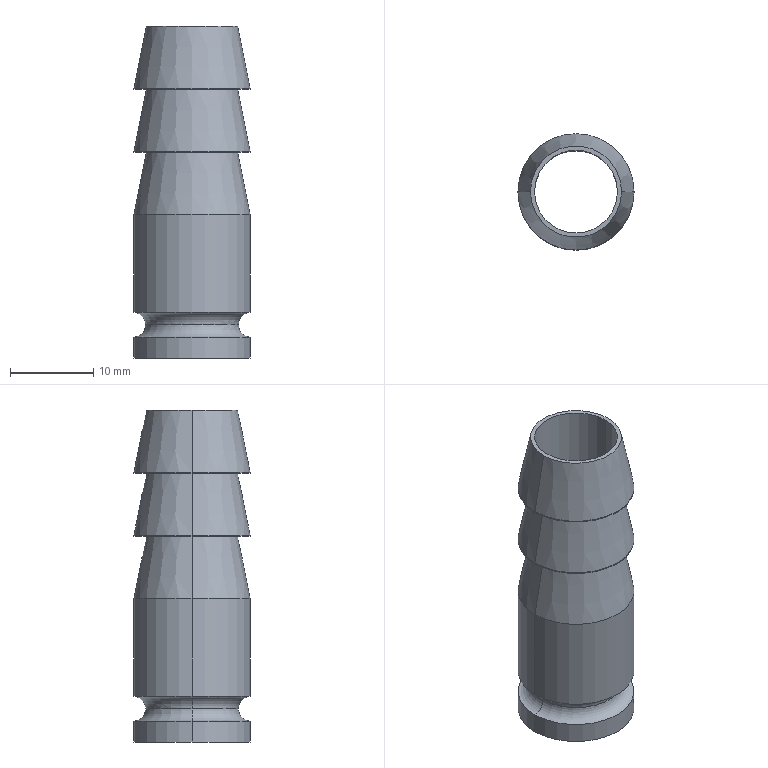Part | STEP file | Air tube connector | 1 solid | 26 faces | box 14 x 14 x 40 mm | volume 2163 mm3 | cylinder 10 | cone 8 | torus 4 | plane 4 | commonest cylinder face diameters 14 x8 10 x2